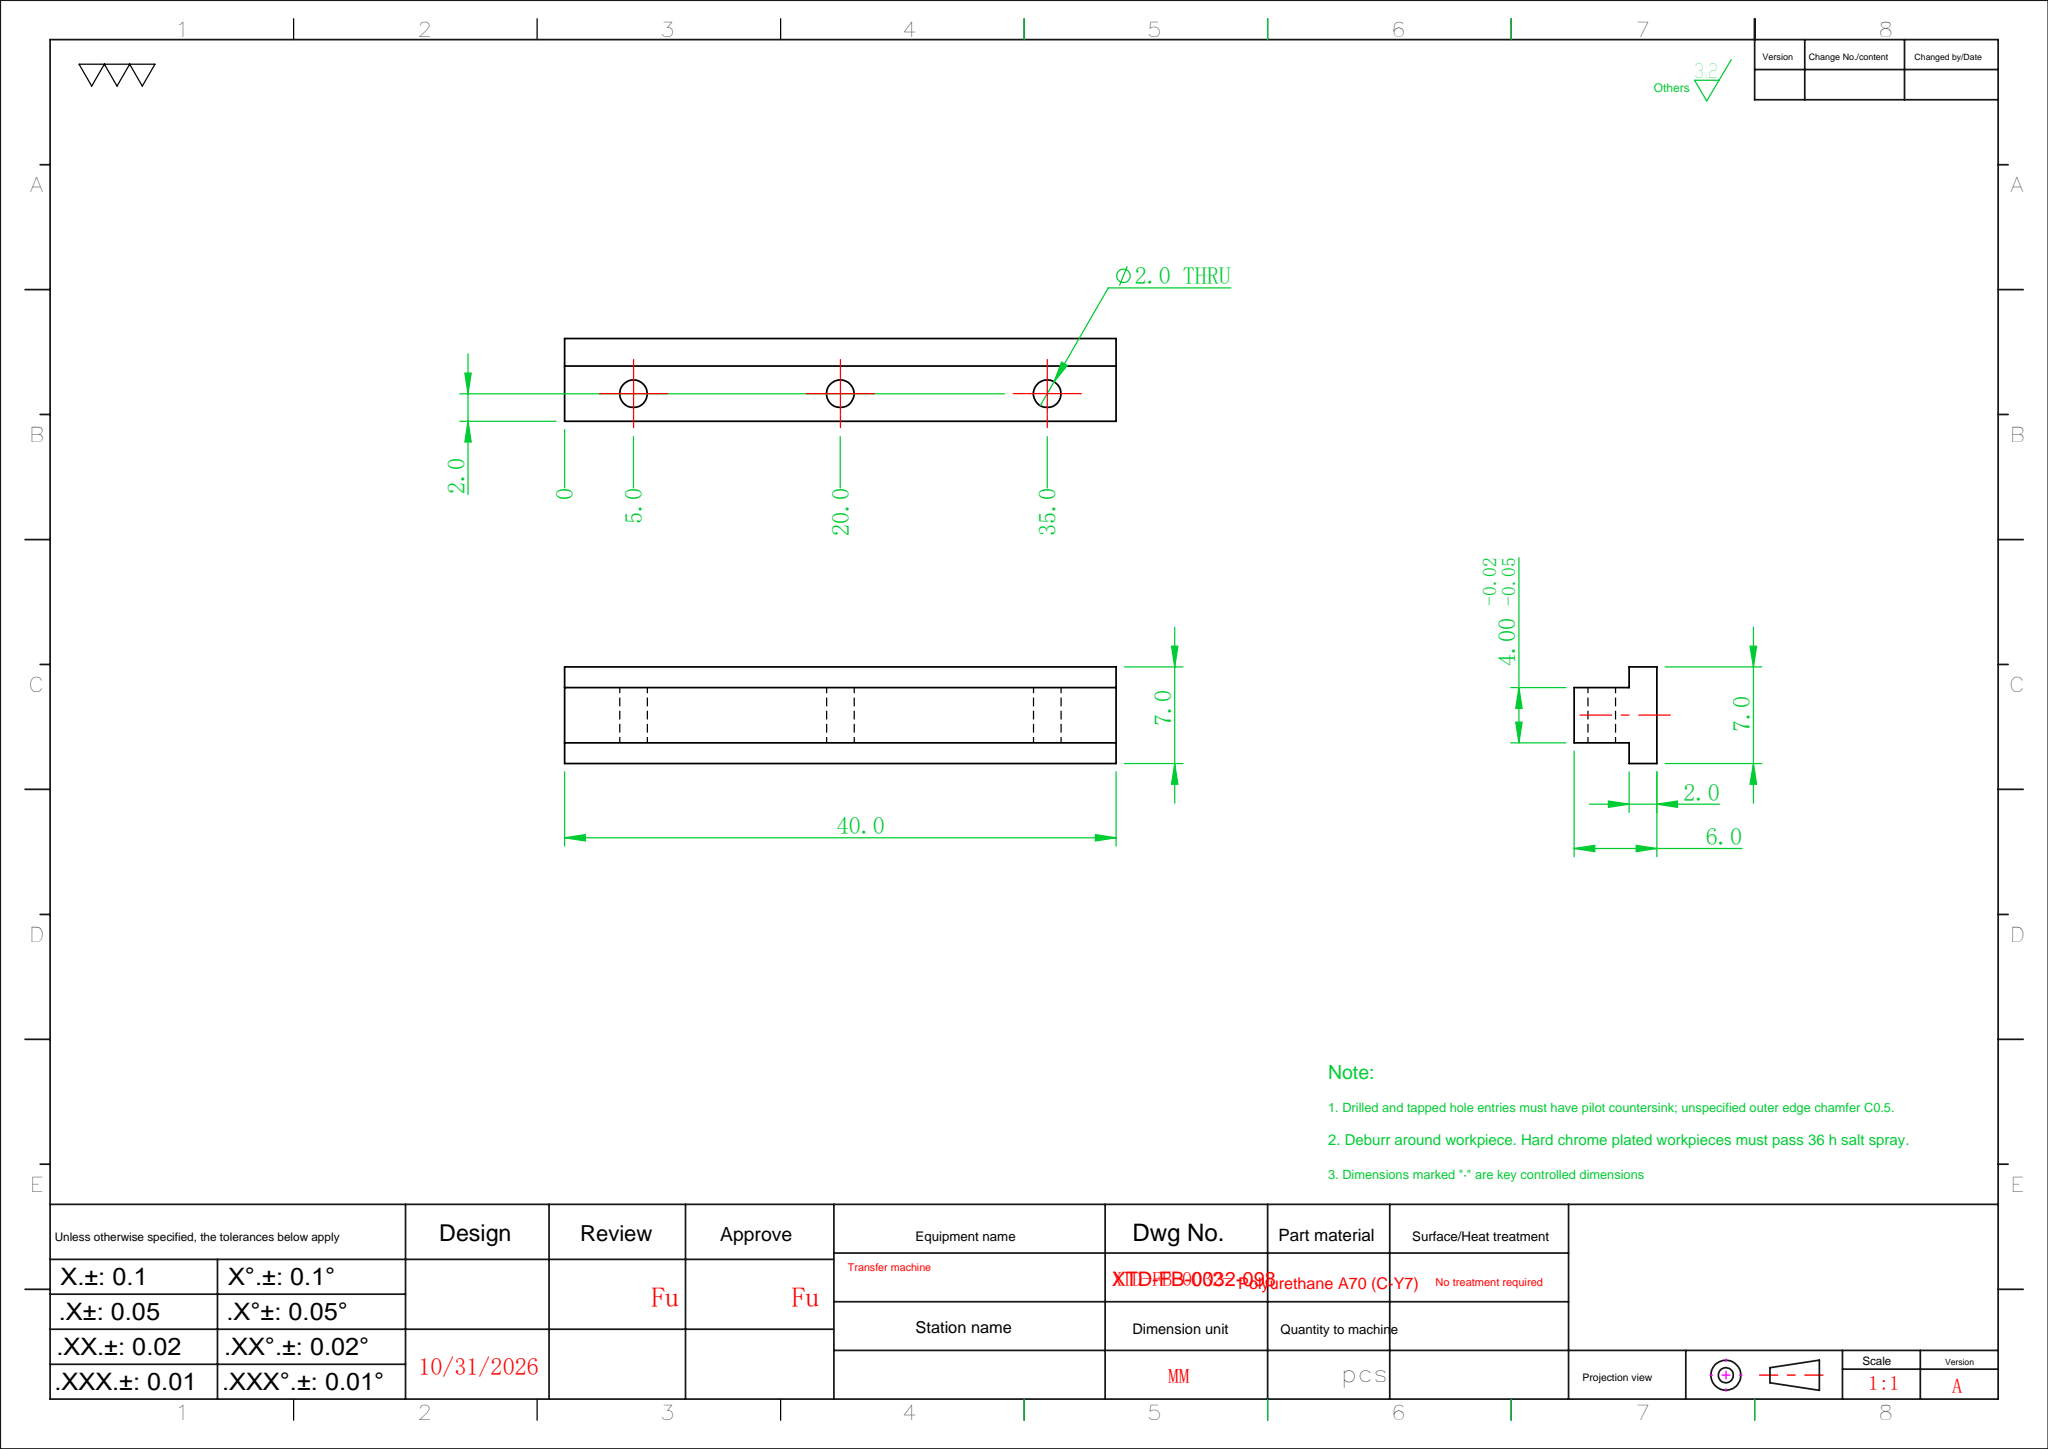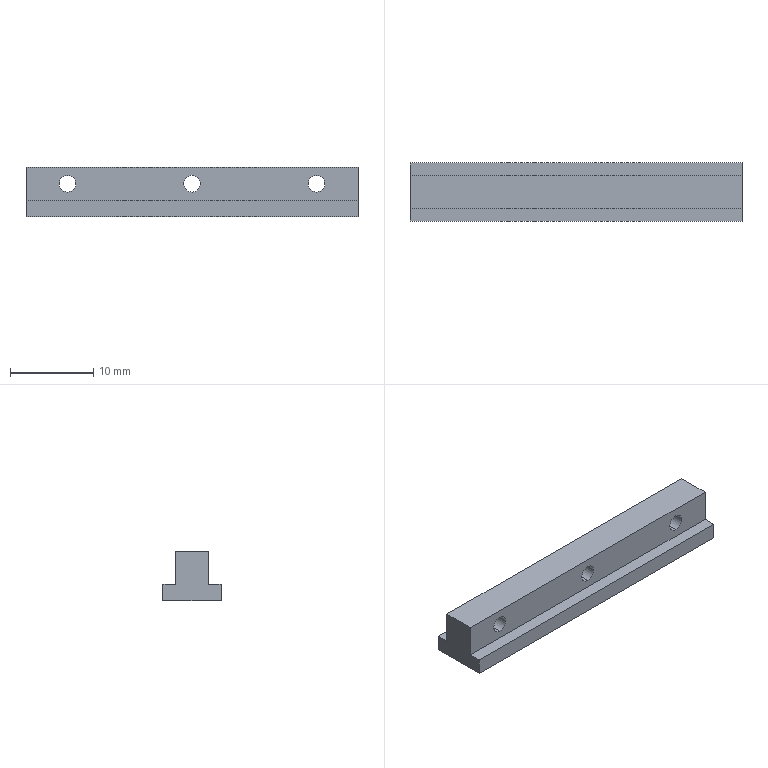Part | SolidWorks | features ICE 2, Extrusion 1 | 1 solid | 16 faces | box 40 x 7 x 6 mm | volume 1162 mm3 | plane 10 | cylinder 6 | commonest cylinder face diameters 2 x6
STEP:
#1=CARTESIAN_POINT('',(-15.,-2.,1.));
#2=VERTEX_POINT('',#1);
#3=CARTESIAN_POINT('',(-15.,-2.,3.));
#4=VERTEX_POINT('',#3);
#5=CARTESIAN_POINT('',(-15.,-2.,2.));
#6=DIRECTION('',(0.,1.,0.));
#7=DIRECTION('',(0.,0.,1.));
#8=AXIS2_PLACEMENT_3D('',#5,#6,#7);
#9=CIRCLE('',#8,1.);
#10=EDGE_CURVE('',#2,#4,#9,.T.);
#11=ORIENTED_EDGE('',*,*,#10,.F.);
#12=CARTESIAN_POINT('',(-15.,2.,1.));
#13=VERTEX_POINT('',#12);
#14=CARTESIAN_POINT('',(-15.,-3.5,1.));
#15=DIRECTION('',(0.,1.,0.));
#16=VECTOR('',#15,1000.);
#17=LINE('',#14,#16);
#18=EDGE_CURVE('',#2,#13,#17,.T.);
#19=ORIENTED_EDGE('',*,*,#18,.T.);
#20=CARTESIAN_POINT('',(-15.,2.,3.));
#21=VERTEX_POINT('',#20);
#22=CARTESIAN_POINT('',(-15.,2.,2.));
#23=DIRECTION('',(0.,1.,0.));
#24=DIRECTION('',(0.,0.,1.));
#25=AXIS2_PLACEMENT_3D('',#22,#23,#24);
#26=CIRCLE('',#25,1.);
#27=EDGE_CURVE('',#13,#21,#26,.T.);
#28=ORIENTED_EDGE('',*,*,#27,.T.);
#29=CARTESIAN_POINT('',(-15.,-3.5,3.));
#30=DIRECTION('',(0.,1.,0.));
#31=VECTOR('',#30,1000.);
#32=LINE('',#29,#31);
#33=EDGE_CURVE('',#4,#21,#32,.T.);
#34=ORIENTED_EDGE('',*,*,#33,.F.);
#35=EDGE_LOOP('',(#11,#19,#28,#34));
#36=FACE_OUTER_BOUND('',#35,.T.);
#37=CARTESIAN_POINT('',(-15.,-3.5,2.));
#38=DIRECTION('',(0.,1.,0.));
#39=DIRECTION('',(0.,0.,1.));
#40=AXIS2_PLACEMENT_3D('',#37,#38,#39);
#41=CYLINDRICAL_SURFACE('',#40,1.);
#42=ADVANCED_FACE('',(#36),#41,.F.);
#43=CARTESIAN_POINT('',(0.,-2.,1.));
#44=VERTEX_POINT('',#43);
#45=CARTESIAN_POINT('',(0.,-2.,3.));
#46=VERTEX_POINT('',#45);
#47=CARTESIAN_POINT('',(0.,-2.,2.));
#48=DIRECTION('',(0.,1.,0.));
#49=DIRECTION('',(0.,0.,1.));
#50=AXIS2_PLACEMENT_3D('',#47,#48,#49);
#51=CIRCLE('',#50,1.);
#52=EDGE_CURVE('',#44,#46,#51,.T.);
#53=ORIENTED_EDGE('',*,*,#52,.F.);
#54=CARTESIAN_POINT('',(0.,2.,1.));
#55=VERTEX_POINT('',#54);
#56=CARTESIAN_POINT('',(0.,-3.5,1.));
#57=DIRECTION('',(0.,1.,0.));
#58=VECTOR('',#57,1000.);
#59=LINE('',#56,#58);
#60=EDGE_CURVE('',#44,#55,#59,.T.);
#61=ORIENTED_EDGE('',*,*,#60,.T.);
#62=CARTESIAN_POINT('',(0.,2.,3.));
#63=VERTEX_POINT('',#62);
#64=CARTESIAN_POINT('',(0.,2.,2.));
#65=DIRECTION('',(0.,1.,0.));
#66=DIRECTION('',(0.,0.,1.));
#67=AXIS2_PLACEMENT_3D('',#64,#65,#66);
#68=CIRCLE('',#67,1.);
#69=EDGE_CURVE('',#55,#63,#68,.T.);
#70=ORIENTED_EDGE('',*,*,#69,.T.);
#71=CARTESIAN_POINT('',(0.,-3.5,3.));
#72=DIRECTION('',(0.,1.,0.));
#73=VECTOR('',#72,1000.);
#74=LINE('',#71,#73);
#75=EDGE_CURVE('',#46,#63,#74,.T.);
#76=ORIENTED_EDGE('',*,*,#75,.F.);
#77=EDGE_LOOP('',(#53,#61,#70,#76));
#78=FACE_OUTER_BOUND('',#77,.T.);
#79=CARTESIAN_POINT('',(0.,-3.5,2.));
#80=DIRECTION('',(0.,1.,0.));
#81=DIRECTION('',(0.,0.,1.));
#82=AXIS2_PLACEMENT_3D('',#79,#80,#81);
#83=CYLINDRICAL_SURFACE('',#82,1.);
#84=ADVANCED_FACE('',(#78),#83,.F.);
#85=CARTESIAN_POINT('',(15.,-2.,1.));
#86=VERTEX_POINT('',#85);
#87=CARTESIAN_POINT('',(15.,-2.,3.));
#88=VERTEX_POINT('',#87);
#89=CARTESIAN_POINT('',(15.,-2.,2.));
#90=DIRECTION('',(0.,1.,0.));
#91=DIRECTION('',(0.,0.,1.));
#92=AXIS2_PLACEMENT_3D('',#89,#90,#91);
#93=CIRCLE('',#92,1.);
#94=EDGE_CURVE('',#86,#88,#93,.T.);
#95=ORIENTED_EDGE('',*,*,#94,.F.);
#96=CARTESIAN_POINT('',(15.,2.,1.));
#97=VERTEX_POINT('',#96);
#98=CARTESIAN_POINT('',(15.,-3.5,1.));
#99=DIRECTION('',(0.,1.,0.));
#100=VECTOR('',#99,1000.);
#101=LINE('',#98,#100);
#102=EDGE_CURVE('',#86,#97,#101,.T.);
#103=ORIENTED_EDGE('',*,*,#102,.T.);
#104=CARTESIAN_POINT('',(15.,2.,3.));
#105=VERTEX_POINT('',#104);
#106=CARTESIAN_POINT('',(15.,2.,2.));
#107=DIRECTION('',(0.,1.,0.));
#108=DIRECTION('',(0.,0.,1.));
#109=AXIS2_PLACEMENT_3D('',#106,#107,#108);
#110=CIRCLE('',#109,1.);
#111=EDGE_CURVE('',#97,#105,#110,.T.);
#112=ORIENTED_EDGE('',*,*,#111,.T.);
#113=CARTESIAN_POINT('',(15.,-3.5,3.));
#114=DIRECTION('',(0.,1.,0.));
#115=VECTOR('',#114,1000.);
#116=LINE('',#113,#115);
#117=EDGE_CURVE('',#88,#105,#116,.T.);
#118=ORIENTED_EDGE('',*,*,#117,.F.);
#119=EDGE_LOOP('',(#95,#103,#112,#118));
#120=FACE_OUTER_BOUND('',#119,.T.);
#121=CARTESIAN_POINT('',(15.,-3.5,2.));
#122=DIRECTION('',(0.,1.,0.));
#123=DIRECTION('',(0.,0.,1.));
#124=AXIS2_PLACEMENT_3D('',#121,#122,#123);
#125=CYLINDRICAL_SURFACE('',#124,1.);
#126=ADVANCED_FACE('',(#120),#125,.F.);
#127=CARTESIAN_POINT('',(20.,-2.,4.));
#128=VERTEX_POINT('',#127);
#129=CARTESIAN_POINT('',(20.,-2.,0.));
#130=VERTEX_POINT('',#129);
#131=CARTESIAN_POINT('',(20.,-2.,4.));
#132=DIRECTION('',(0.,0.,-1.));
#133=VECTOR('',#132,1000.);
#134=LINE('',#131,#133);
#135=EDGE_CURVE('',#128,#130,#134,.T.);
#136=ORIENTED_EDGE('',*,*,#135,.T.);
#137=CARTESIAN_POINT('',(20.,-3.5,0.));
#138=VERTEX_POINT('',#137);
#139=CARTESIAN_POINT('',(20.,-3.5,0.));
#140=DIRECTION('',(0.,-1.,0.));
#141=VECTOR('',#140,1000.);
#142=LINE('',#139,#141);
#143=EDGE_CURVE('',#130,#138,#142,.T.);
#144=ORIENTED_EDGE('',*,*,#143,.T.);
#145=CARTESIAN_POINT('',(20.,-3.5,-2.));
#146=VERTEX_POINT('',#145);
#147=CARTESIAN_POINT('',(20.,-3.5,0.));
#148=DIRECTION('',(0.,0.,-1.));
#149=VECTOR('',#148,1000.);
#150=LINE('',#147,#149);
#151=EDGE_CURVE('',#138,#146,#150,.T.);
#152=ORIENTED_EDGE('',*,*,#151,.T.);
#153=CARTESIAN_POINT('',(20.,3.5,-2.));
#154=VERTEX_POINT('',#153);
#155=CARTESIAN_POINT('',(20.,-3.5,-2.));
#156=DIRECTION('',(0.,1.,0.));
#157=VECTOR('',#156,1000.);
#158=LINE('',#155,#157);
#159=EDGE_CURVE('',#146,#154,#158,.T.);
#160=ORIENTED_EDGE('',*,*,#159,.T.);
#161=CARTESIAN_POINT('',(20.,3.5,0.));
#162=VERTEX_POINT('',#161);
#163=CARTESIAN_POINT('',(20.,3.5,0.));
#164=DIRECTION('',(0.,0.,1.));
#165=VECTOR('',#164,1000.);
#166=LINE('',#163,#165);
#167=EDGE_CURVE('',#154,#162,#166,.T.);
#168=ORIENTED_EDGE('',*,*,#167,.T.);
#169=CARTESIAN_POINT('',(20.,2.,0.));
#170=VERTEX_POINT('',#169);
#171=CARTESIAN_POINT('',(20.,-3.5,0.));
#172=DIRECTION('',(0.,-1.,0.));
#173=VECTOR('',#172,1000.);
#174=LINE('',#171,#173);
#175=EDGE_CURVE('',#162,#170,#174,.T.);
#176=ORIENTED_EDGE('',*,*,#175,.T.);
#177=CARTESIAN_POINT('',(20.,2.,4.));
#178=VERTEX_POINT('',#177);
#179=CARTESIAN_POINT('',(20.,2.,4.));
#180=DIRECTION('',(0.,0.,-1.));
#181=VECTOR('',#180,1000.);
#182=LINE('',#179,#181);
#183=EDGE_CURVE('',#178,#170,#182,.T.);
#184=ORIENTED_EDGE('',*,*,#183,.F.);
#185=CARTESIAN_POINT('',(20.,-2.,4.));
#186=DIRECTION('',(0.,1.,0.));
#187=VECTOR('',#186,1000.);
#188=LINE('',#185,#187);
#189=EDGE_CURVE('',#128,#178,#188,.T.);
#190=ORIENTED_EDGE('',*,*,#189,.F.);
#191=EDGE_LOOP('',(#136,#144,#152,#160,#168,#176,#184,#190));
#192=FACE_OUTER_BOUND('',#191,.T.);
#193=CARTESIAN_POINT('',(20.,-2.,4.));
#194=DIRECTION('',(-1.,0.,0.));
#195=DIRECTION('',(0.,0.,1.));
#196=AXIS2_PLACEMENT_3D('',#193,#194,#195);
#197=PLANE('',#196);
#198=ADVANCED_FACE('',(#192),#197,.F.);
#199=CARTESIAN_POINT('',(-15.,2.,2.));
#200=DIRECTION('',(0.,1.,0.));
#201=DIRECTION('',(0.,0.,1.));
#202=AXIS2_PLACEMENT_3D('',#199,#200,#201);
#203=CIRCLE('',#202,1.);
#204=EDGE_CURVE('',#21,#13,#203,.T.);
#205=ORIENTED_EDGE('',*,*,#204,.F.);
#206=ORIENTED_EDGE('',*,*,#27,.F.);
#207=EDGE_LOOP('',(#205,#206));
#208=FACE_BOUND('',#207,.T.);
#209=CARTESIAN_POINT('',(0.,2.,2.));
#210=DIRECTION('',(0.,1.,0.));
#211=DIRECTION('',(0.,0.,1.));
#212=AXIS2_PLACEMENT_3D('',#209,#210,#211);
#213=CIRCLE('',#212,1.);
#214=EDGE_CURVE('',#63,#55,#213,.T.);
#215=ORIENTED_EDGE('',*,*,#214,.F.);
#216=ORIENTED_EDGE('',*,*,#69,.F.);
#217=EDGE_LOOP('',(#215,#216));
#218=FACE_BOUND('',#217,.T.);
#219=CARTESIAN_POINT('',(15.,2.,2.));
#220=DIRECTION('',(0.,1.,0.));
#221=DIRECTION('',(0.,0.,1.));
#222=AXIS2_PLACEMENT_3D('',#219,#220,#221);
#223=CIRCLE('',#222,1.);
#224=EDGE_CURVE('',#105,#97,#223,.T.);
#225=ORIENTED_EDGE('',*,*,#224,.F.);
#226=ORIENTED_EDGE('',*,*,#111,.F.);
#227=EDGE_LOOP('',(#225,#226));
#228=FACE_BOUND('',#227,.T.);
#229=CARTESIAN_POINT('',(-20.,2.,0.));
#230=VERTEX_POINT('',#229);
#231=CARTESIAN_POINT('',(-20.,2.,0.));
#232=DIRECTION('',(-1.,0.,0.));
#233=VECTOR('',#232,1000.);
#234=LINE('',#231,#233);
#235=EDGE_CURVE('',#170,#230,#234,.T.);
#236=ORIENTED_EDGE('',*,*,#235,.T.);
#237=CARTESIAN_POINT('',(-20.,2.,4.));
#238=VERTEX_POINT('',#237);
#239=CARTESIAN_POINT('',(-20.,2.,4.));
#240=DIRECTION('',(0.,0.,-1.));
#241=VECTOR('',#240,1000.);
#242=LINE('',#239,#241);
#243=EDGE_CURVE('',#238,#230,#242,.T.);
#244=ORIENTED_EDGE('',*,*,#243,.F.);
#245=CARTESIAN_POINT('',(-20.,2.,4.));
#246=DIRECTION('',(-1.,0.,0.));
#247=VECTOR('',#246,1000.);
#248=LINE('',#245,#247);
#249=EDGE_CURVE('',#178,#238,#248,.T.);
#250=ORIENTED_EDGE('',*,*,#249,.F.);
#251=ORIENTED_EDGE('',*,*,#183,.T.);
#252=EDGE_LOOP('',(#236,#244,#250,#251));
#253=FACE_OUTER_BOUND('',#252,.T.);
#254=CARTESIAN_POINT('',(-20.,2.,4.));
#255=DIRECTION('',(0.,-1.,0.));
#256=DIRECTION('',(0.,0.,-1.));
#257=AXIS2_PLACEMENT_3D('',#254,#255,#256);
#258=PLANE('',#257);
#259=ADVANCED_FACE('',(#208,#218,#228,#253),#258,.F.);
#260=ORIENTED_EDGE('',*,*,#243,.T.);
#261=CARTESIAN_POINT('',(-20.,3.5,0.));
#262=VERTEX_POINT('',#261);
#263=CARTESIAN_POINT('',(-20.,-3.5,0.));
#264=DIRECTION('',(0.,1.,0.));
#265=VECTOR('',#264,1000.);
#266=LINE('',#263,#265);
#267=EDGE_CURVE('',#230,#262,#266,.T.);
#268=ORIENTED_EDGE('',*,*,#267,.T.);
#269=CARTESIAN_POINT('',(-20.,3.5,-2.));
#270=VERTEX_POINT('',#269);
#271=CARTESIAN_POINT('',(-20.,3.5,0.));
#272=DIRECTION('',(0.,0.,-1.));
#273=VECTOR('',#272,1000.);
#274=LINE('',#271,#273);
#275=EDGE_CURVE('',#262,#270,#274,.T.);
#276=ORIENTED_EDGE('',*,*,#275,.T.);
#277=CARTESIAN_POINT('',(-20.,-3.5,-2.));
#278=VERTEX_POINT('',#277);
#279=CARTESIAN_POINT('',(-20.,-3.5,-2.));
#280=DIRECTION('',(0.,-1.,0.));
#281=VECTOR('',#280,1000.);
#282=LINE('',#279,#281);
#283=EDGE_CURVE('',#270,#278,#282,.T.);
#284=ORIENTED_EDGE('',*,*,#283,.T.);
#285=CARTESIAN_POINT('',(-20.,-3.5,0.));
#286=VERTEX_POINT('',#285);
#287=CARTESIAN_POINT('',(-20.,-3.5,0.));
#288=DIRECTION('',(0.,0.,1.));
#289=VECTOR('',#288,1000.);
#290=LINE('',#287,#289);
#291=EDGE_CURVE('',#278,#286,#290,.T.);
#292=ORIENTED_EDGE('',*,*,#291,.T.);
#293=CARTESIAN_POINT('',(-20.,-2.,0.));
#294=VERTEX_POINT('',#293);
#295=CARTESIAN_POINT('',(-20.,-3.5,0.));
#296=DIRECTION('',(0.,1.,0.));
#297=VECTOR('',#296,1000.);
#298=LINE('',#295,#297);
#299=EDGE_CURVE('',#286,#294,#298,.T.);
#300=ORIENTED_EDGE('',*,*,#299,.T.);
#301=CARTESIAN_POINT('',(-20.,-2.,4.));
#302=VERTEX_POINT('',#301);
#303=CARTESIAN_POINT('',(-20.,-2.,4.));
#304=DIRECTION('',(0.,0.,-1.));
#305=VECTOR('',#304,1000.);
#306=LINE('',#303,#305);
#307=EDGE_CURVE('',#302,#294,#306,.T.);
#308=ORIENTED_EDGE('',*,*,#307,.F.);
#309=CARTESIAN_POINT('',(-20.,-2.,4.));
#310=DIRECTION('',(0.,-1.,0.));
#311=VECTOR('',#310,1000.);
#312=LINE('',#309,#311);
#313=EDGE_CURVE('',#238,#302,#312,.T.);
#314=ORIENTED_EDGE('',*,*,#313,.F.);
#315=EDGE_LOOP('',(#260,#268,#276,#284,#292,#300,#308,#314));
#316=FACE_OUTER_BOUND('',#315,.T.);
#317=CARTESIAN_POINT('',(-20.,-2.,4.));
#318=DIRECTION('',(1.,0.,0.));
#319=DIRECTION('',(0.,0.,-1.));
#320=AXIS2_PLACEMENT_3D('',#317,#318,#319);
#321=PLANE('',#320);
#322=ADVANCED_FACE('',(#316),#321,.F.);
#323=CARTESIAN_POINT('',(-15.,-2.,2.));
#324=DIRECTION('',(0.,1.,0.));
#325=DIRECTION('',(0.,0.,1.));
#326=AXIS2_PLACEMENT_3D('',#323,#324,#325);
#327=CIRCLE('',#326,1.);
#328=EDGE_CURVE('',#4,#2,#327,.T.);
#329=ORIENTED_EDGE('',*,*,#328,.T.);
#330=ORIENTED_EDGE('',*,*,#10,.T.);
#331=EDGE_LOOP('',(#329,#330));
#332=FACE_BOUND('',#331,.T.);
#333=CARTESIAN_POINT('',(0.,-2.,2.));
#334=DIRECTION('',(0.,1.,0.));
#335=DIRECTION('',(0.,0.,1.));
#336=AXIS2_PLACEMENT_3D('',#333,#334,#335);
#337=CIRCLE('',#336,1.);
#338=EDGE_CURVE('',#46,#44,#337,.T.);
#339=ORIENTED_EDGE('',*,*,#338,.T.);
#340=ORIENTED_EDGE('',*,*,#52,.T.);
#341=EDGE_LOOP('',(#339,#340));
#342=FACE_BOUND('',#341,.T.);
#343=CARTESIAN_POINT('',(15.,-2.,2.));
#344=DIRECTION('',(0.,1.,0.));
#345=DIRECTION('',(0.,0.,1.));
#346=AXIS2_PLACEMENT_3D('',#343,#344,#345);
#347=CIRCLE('',#346,1.);
#348=EDGE_CURVE('',#88,#86,#347,.T.);
#349=ORIENTED_EDGE('',*,*,#348,.T.);
#350=ORIENTED_EDGE('',*,*,#94,.T.);
#351=EDGE_LOOP('',(#349,#350));
#352=FACE_BOUND('',#351,.T.);
#353=CARTESIAN_POINT('',(-20.,-2.,0.));
#354=DIRECTION('',(1.,0.,0.));
#355=VECTOR('',#354,1000.);
#356=LINE('',#353,#355);
#357=EDGE_CURVE('',#294,#130,#356,.T.);
#358=ORIENTED_EDGE('',*,*,#357,.T.);
#359=ORIENTED_EDGE('',*,*,#135,.F.);
#360=CARTESIAN_POINT('',(-20.,-2.,4.));
#361=DIRECTION('',(1.,0.,0.));
#362=VECTOR('',#361,1000.);
#363=LINE('',#360,#362);
#364=EDGE_CURVE('',#302,#128,#363,.T.);
#365=ORIENTED_EDGE('',*,*,#364,.F.);
#366=ORIENTED_EDGE('',*,*,#307,.T.);
#367=EDGE_LOOP('',(#358,#359,#365,#366));
#368=FACE_OUTER_BOUND('',#367,.T.);
#369=CARTESIAN_POINT('',(-20.,-2.,4.));
#370=DIRECTION('',(0.,1.,0.));
#371=DIRECTION('',(0.,0.,1.));
#372=AXIS2_PLACEMENT_3D('',#369,#370,#371);
#373=PLANE('',#372);
#374=ADVANCED_FACE('',(#332,#342,#352,#368),#373,.F.);
#375=ORIENTED_EDGE('',*,*,#189,.T.);
#376=ORIENTED_EDGE('',*,*,#249,.T.);
#377=ORIENTED_EDGE('',*,*,#313,.T.);
#378=ORIENTED_EDGE('',*,*,#364,.T.);
#379=EDGE_LOOP('',(#375,#376,#377,#378));
#380=FACE_OUTER_BOUND('',#379,.T.);
#381=CARTESIAN_POINT('',(0.,0.,4.));
#382=DIRECTION('',(0.,0.,-1.));
#383=DIRECTION('',(-1.,0.,0.));
#384=AXIS2_PLACEMENT_3D('',#381,#382,#383);
#385=PLANE('',#384);
#386=ADVANCED_FACE('',(#380),#385,.F.);
#387=ORIENTED_EDGE('',*,*,#357,.F.);
#388=ORIENTED_EDGE('',*,*,#299,.F.);
#389=CARTESIAN_POINT('',(-27.28,-3.5,0.));
#390=DIRECTION('',(1.,0.,0.));
#391=VECTOR('',#390,1000.);
#392=LINE('',#389,#391);
#393=EDGE_CURVE('',#286,#138,#392,.T.);
#394=ORIENTED_EDGE('',*,*,#393,.T.);
#395=ORIENTED_EDGE('',*,*,#143,.F.);
#396=EDGE_LOOP('',(#387,#388,#394,#395));
#397=FACE_OUTER_BOUND('',#396,.T.);
#398=CARTESIAN_POINT('',(-27.28,-3.5,0.));
#399=DIRECTION('',(0.,0.,1.));
#400=DIRECTION('',(1.,0.,0.));
#401=AXIS2_PLACEMENT_3D('',#398,#399,#400);
#402=PLANE('',#401);
#403=ADVANCED_FACE('',(#397),#402,.T.);
#404=ORIENTED_EDGE('',*,*,#235,.F.);
#405=ORIENTED_EDGE('',*,*,#175,.F.);
#406=CARTESIAN_POINT('',(-27.28,3.5,0.));
#407=DIRECTION('',(1.,0.,0.));
#408=VECTOR('',#407,1000.);
#409=LINE('',#406,#408);
#410=EDGE_CURVE('',#262,#162,#409,.T.);
#411=ORIENTED_EDGE('',*,*,#410,.F.);
#412=ORIENTED_EDGE('',*,*,#267,.F.);
#413=EDGE_LOOP('',(#404,#405,#411,#412));
#414=FACE_OUTER_BOUND('',#413,.T.);
#415=CARTESIAN_POINT('',(-27.28,-3.5,0.));
#416=DIRECTION('',(0.,0.,1.));
#417=DIRECTION('',(1.,0.,0.));
#418=AXIS2_PLACEMENT_3D('',#415,#416,#417);
#419=PLANE('',#418);
#420=ADVANCED_FACE('',(#414),#419,.T.);
#421=ORIENTED_EDGE('',*,*,#275,.F.);
#422=ORIENTED_EDGE('',*,*,#410,.T.);
#423=ORIENTED_EDGE('',*,*,#167,.F.);
#424=CARTESIAN_POINT('',(-27.28,3.5,-2.));
#425=DIRECTION('',(1.,0.,0.));
#426=VECTOR('',#425,1000.);
#427=LINE('',#424,#426);
#428=EDGE_CURVE('',#270,#154,#427,.T.);
#429=ORIENTED_EDGE('',*,*,#428,.F.);
#430=EDGE_LOOP('',(#421,#422,#423,#429));
#431=FACE_OUTER_BOUND('',#430,.T.);
#432=CARTESIAN_POINT('',(-27.28,3.5,0.));
#433=DIRECTION('',(0.,1.,0.));
#434=DIRECTION('',(0.,0.,1.));
#435=AXIS2_PLACEMENT_3D('',#432,#433,#434);
#436=PLANE('',#435);
#437=ADVANCED_FACE('',(#431),#436,.T.);
#438=ORIENTED_EDGE('',*,*,#283,.F.);
#439=ORIENTED_EDGE('',*,*,#428,.T.);
#440=ORIENTED_EDGE('',*,*,#159,.F.);
#441=CARTESIAN_POINT('',(-27.28,-3.5,-2.));
#442=DIRECTION('',(1.,0.,0.));
#443=VECTOR('',#442,1000.);
#444=LINE('',#441,#443);
#445=EDGE_CURVE('',#278,#146,#444,.T.);
#446=ORIENTED_EDGE('',*,*,#445,.F.);
#447=EDGE_LOOP('',(#438,#439,#440,#446));
#448=FACE_OUTER_BOUND('',#447,.T.);
#449=CARTESIAN_POINT('',(-27.28,-3.5,-2.));
#450=DIRECTION('',(0.,0.,-1.));
#451=DIRECTION('',(-1.,0.,0.));
#452=AXIS2_PLACEMENT_3D('',#449,#450,#451);
#453=PLANE('',#452);
#454=ADVANCED_FACE('',(#448),#453,.T.);
#455=ORIENTED_EDGE('',*,*,#291,.F.);
#456=ORIENTED_EDGE('',*,*,#445,.T.);
#457=ORIENTED_EDGE('',*,*,#151,.F.);
#458=ORIENTED_EDGE('',*,*,#393,.F.);
#459=EDGE_LOOP('',(#455,#456,#457,#458));
#460=FACE_OUTER_BOUND('',#459,.T.);
#461=CARTESIAN_POINT('',(-27.28,-3.5,0.));
#462=DIRECTION('',(0.,-1.,0.));
#463=DIRECTION('',(0.,0.,-1.));
#464=AXIS2_PLACEMENT_3D('',#461,#462,#463);
#465=PLANE('',#464);
#466=ADVANCED_FACE('',(#460),#465,.T.);
#467=ORIENTED_EDGE('',*,*,#102,.F.);
#468=ORIENTED_EDGE('',*,*,#348,.F.);
#469=ORIENTED_EDGE('',*,*,#117,.T.);
#470=ORIENTED_EDGE('',*,*,#224,.T.);
#471=EDGE_LOOP('',(#467,#468,#469,#470));
#472=FACE_OUTER_BOUND('',#471,.T.);
#473=CARTESIAN_POINT('',(15.,-3.5,2.));
#474=DIRECTION('',(0.,1.,0.));
#475=DIRECTION('',(0.,0.,1.));
#476=AXIS2_PLACEMENT_3D('',#473,#474,#475);
#477=CYLINDRICAL_SURFACE('',#476,1.);
#478=ADVANCED_FACE('',(#472),#477,.F.);
#479=ORIENTED_EDGE('',*,*,#60,.F.);
#480=ORIENTED_EDGE('',*,*,#338,.F.);
#481=ORIENTED_EDGE('',*,*,#75,.T.);
#482=ORIENTED_EDGE('',*,*,#214,.T.);
#483=EDGE_LOOP('',(#479,#480,#481,#482));
#484=FACE_OUTER_BOUND('',#483,.T.);
#485=CARTESIAN_POINT('',(0.,-3.5,2.));
#486=DIRECTION('',(0.,1.,0.));
#487=DIRECTION('',(0.,0.,1.));
#488=AXIS2_PLACEMENT_3D('',#485,#486,#487);
#489=CYLINDRICAL_SURFACE('',#488,1.);
#490=ADVANCED_FACE('',(#484),#489,.F.);
#491=ORIENTED_EDGE('',*,*,#18,.F.);
#492=ORIENTED_EDGE('',*,*,#328,.F.);
#493=ORIENTED_EDGE('',*,*,#33,.T.);
#494=ORIENTED_EDGE('',*,*,#204,.T.);
#495=EDGE_LOOP('',(#491,#492,#493,#494));
#496=FACE_OUTER_BOUND('',#495,.T.);
#497=CARTESIAN_POINT('',(-15.,-3.5,2.));
#498=DIRECTION('',(0.,1.,0.));
#499=DIRECTION('',(0.,0.,1.));
#500=AXIS2_PLACEMENT_3D('',#497,#498,#499);
#501=CYLINDRICAL_SURFACE('',#500,1.);
#502=ADVANCED_FACE('',(#496),#501,.F.);
#503=CLOSED_SHELL('',(#42,#84,#126,#198,#259,#322,#374,#386,#403,#420,#437,#454,#466,#478,#490,#502));
#504=MANIFOLD_SOLID_BREP('',#503);
#505=CARTESIAN_POINT('',(0.,0.,0.));
#506=DIRECTION('',(0.,0.,1.));
#507=DIRECTION('',(1.,0.,0.));
#508=AXIS2_PLACEMENT_3D('',#505,#506,#507);
#509=(LENGTH_UNIT()NAMED_UNIT(*)SI_UNIT(.MILLI.,.METRE.));
#510=UNCERTAINTY_MEASURE_WITH_UNIT(LENGTH_MEASURE(0.00001),#509,'','');
#511=(NAMED_UNIT(*)PLANE_ANGLE_UNIT()SI_UNIT($,.RADIAN.));
#512=(NAMED_UNIT(*)SI_UNIT($,.STERADIAN.)SOLID_ANGLE_UNIT());
#513=(GEOMETRIC_REPRESENTATION_CONTEXT(3)GLOBAL_UNCERTAINTY_ASSIGNED_CONTEXT((#510))GLOBAL_UNIT_ASSIGNED_CONTEXT((#509,#511,#512))REPRESENTATION_CONTEXT('',''));
#514=ADVANCED_BREP_SHAPE_REPRESENTATION('',(#504,#508),#513);